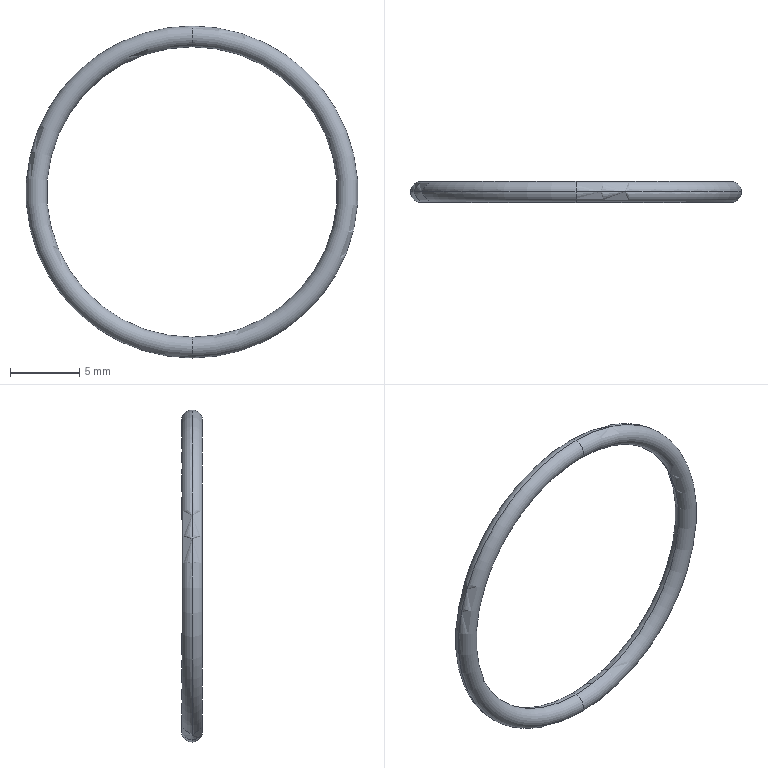Part | SolidWorks | features Revolution 1 | 1 solid | 4 faces | box 24 x 1.5 x 24 mm | volume 124.912 mm3 | torus 4
STEP:
#1=CARTESIAN_POINT('',(0.,0.,12.));
#2=VERTEX_POINT('',#1);
#3=CARTESIAN_POINT('',(0.,0.,10.5));
#4=VERTEX_POINT('',#3);
#5=CARTESIAN_POINT('',(0.,0.,11.25));
#6=DIRECTION('',(1.,0.,0.));
#7=DIRECTION('',(0.,0.,-1.));
#8=AXIS2_PLACEMENT_3D('',#5,#6,#7);
#9=CIRCLE('',#8,0.75);
#10=EDGE_CURVE('',#2,#4,#9,.T.);
#11=ORIENTED_EDGE('',*,*,#10,.F.);
#12=CARTESIAN_POINT('',(0.,0.,-12.));
#13=VERTEX_POINT('',#12);
#14=CARTESIAN_POINT('',(0.,0.,0.));
#15=DIRECTION('',(0.,-1.,0.));
#16=DIRECTION('',(0.,0.,-1.));
#17=AXIS2_PLACEMENT_3D('',#14,#15,#16);
#18=CIRCLE('',#17,12.);
#19=EDGE_CURVE('',#2,#13,#18,.T.);
#20=ORIENTED_EDGE('',*,*,#19,.T.);
#21=CARTESIAN_POINT('',(0.,0.,-10.5));
#22=VERTEX_POINT('',#21);
#23=CARTESIAN_POINT('',(0.,0.,-11.25));
#24=DIRECTION('',(-1.,0.,0.));
#25=DIRECTION('',(0.,0.,1.));
#26=AXIS2_PLACEMENT_3D('',#23,#24,#25);
#27=CIRCLE('',#26,0.75);
#28=EDGE_CURVE('',#13,#22,#27,.T.);
#29=ORIENTED_EDGE('',*,*,#28,.T.);
#30=CARTESIAN_POINT('',(0.,0.,0.));
#31=DIRECTION('',(0.,-1.,0.));
#32=DIRECTION('',(0.,0.,-1.));
#33=AXIS2_PLACEMENT_3D('',#30,#31,#32);
#34=CIRCLE('',#33,10.5);
#35=EDGE_CURVE('',#4,#22,#34,.T.);
#36=ORIENTED_EDGE('',*,*,#35,.F.);
#37=EDGE_LOOP('',(#11,#20,#29,#36));
#38=FACE_OUTER_BOUND('',#37,.T.);
#39=CARTESIAN_POINT('',(0.,0.,0.));
#40=DIRECTION('',(0.,-1.,0.));
#41=DIRECTION('',(0.,0.,-1.));
#42=AXIS2_PLACEMENT_3D('',#39,#40,#41);
#43=TOROIDAL_SURFACE('',#42,11.25,0.75);
#44=ADVANCED_FACE('',(#38),#43,.T.);
#45=ORIENTED_EDGE('',*,*,#28,.F.);
#46=CARTESIAN_POINT('',(0.,0.,0.));
#47=DIRECTION('',(0.,-1.,0.));
#48=DIRECTION('',(0.,0.,-1.));
#49=AXIS2_PLACEMENT_3D('',#46,#47,#48);
#50=CIRCLE('',#49,12.);
#51=EDGE_CURVE('',#13,#2,#50,.T.);
#52=ORIENTED_EDGE('',*,*,#51,.T.);
#53=ORIENTED_EDGE('',*,*,#10,.T.);
#54=CARTESIAN_POINT('',(0.,0.,0.));
#55=DIRECTION('',(0.,-1.,0.));
#56=DIRECTION('',(0.,0.,-1.));
#57=AXIS2_PLACEMENT_3D('',#54,#55,#56);
#58=CIRCLE('',#57,10.5);
#59=EDGE_CURVE('',#22,#4,#58,.T.);
#60=ORIENTED_EDGE('',*,*,#59,.F.);
#61=EDGE_LOOP('',(#45,#52,#53,#60));
#62=FACE_OUTER_BOUND('',#61,.T.);
#63=CARTESIAN_POINT('',(0.,0.,0.));
#64=DIRECTION('',(0.,-1.,0.));
#65=DIRECTION('',(0.,0.,-1.));
#66=AXIS2_PLACEMENT_3D('',#63,#64,#65);
#67=TOROIDAL_SURFACE('',#66,11.25,0.75);
#68=ADVANCED_FACE('',(#62),#67,.T.);
#69=ORIENTED_EDGE('',*,*,#51,.F.);
#70=CARTESIAN_POINT('',(0.,0.,-11.25));
#71=DIRECTION('',(-1.,0.,0.));
#72=DIRECTION('',(0.,0.,1.));
#73=AXIS2_PLACEMENT_3D('',#70,#71,#72);
#74=CIRCLE('',#73,0.75);
#75=EDGE_CURVE('',#22,#13,#74,.T.);
#76=ORIENTED_EDGE('',*,*,#75,.F.);
#77=ORIENTED_EDGE('',*,*,#59,.T.);
#78=CARTESIAN_POINT('',(0.,0.,11.25));
#79=DIRECTION('',(1.,0.,0.));
#80=DIRECTION('',(0.,0.,-1.));
#81=AXIS2_PLACEMENT_3D('',#78,#79,#80);
#82=CIRCLE('',#81,0.75);
#83=EDGE_CURVE('',#4,#2,#82,.T.);
#84=ORIENTED_EDGE('',*,*,#83,.T.);
#85=EDGE_LOOP('',(#69,#76,#77,#84));
#86=FACE_OUTER_BOUND('',#85,.T.);
#87=CARTESIAN_POINT('',(0.,0.,0.));
#88=DIRECTION('',(0.,-1.,0.));
#89=DIRECTION('',(0.,0.,-1.));
#90=AXIS2_PLACEMENT_3D('',#87,#88,#89);
#91=TOROIDAL_SURFACE('',#90,11.25,0.75);
#92=ADVANCED_FACE('',(#86),#91,.T.);
#93=ORIENTED_EDGE('',*,*,#19,.F.);
#94=ORIENTED_EDGE('',*,*,#83,.F.);
#95=ORIENTED_EDGE('',*,*,#35,.T.);
#96=ORIENTED_EDGE('',*,*,#75,.T.);
#97=EDGE_LOOP('',(#93,#94,#95,#96));
#98=FACE_OUTER_BOUND('',#97,.T.);
#99=CARTESIAN_POINT('',(0.,0.,0.));
#100=DIRECTION('',(0.,-1.,0.));
#101=DIRECTION('',(0.,0.,-1.));
#102=AXIS2_PLACEMENT_3D('',#99,#100,#101);
#103=TOROIDAL_SURFACE('',#102,11.25,0.75);
#104=ADVANCED_FACE('',(#98),#103,.T.);
#105=CLOSED_SHELL('',(#44,#68,#92,#104));
#106=MANIFOLD_SOLID_BREP('',#105);
#107=CARTESIAN_POINT('',(0.,0.,0.));
#108=DIRECTION('',(0.,0.,1.));
#109=DIRECTION('',(1.,0.,0.));
#110=AXIS2_PLACEMENT_3D('',#107,#108,#109);
#111=(LENGTH_UNIT()NAMED_UNIT(*)SI_UNIT(.MILLI.,.METRE.));
#112=UNCERTAINTY_MEASURE_WITH_UNIT(LENGTH_MEASURE(0.00001),#111,'','');
#113=(NAMED_UNIT(*)PLANE_ANGLE_UNIT()SI_UNIT($,.RADIAN.));
#114=(NAMED_UNIT(*)SI_UNIT($,.STERADIAN.)SOLID_ANGLE_UNIT());
#115=(GEOMETRIC_REPRESENTATION_CONTEXT(3)GLOBAL_UNCERTAINTY_ASSIGNED_CONTEXT((#112))GLOBAL_UNIT_ASSIGNED_CONTEXT((#111,#113,#114))REPRESENTATION_CONTEXT('',''));
#116=ADVANCED_BREP_SHAPE_REPRESENTATION('',(#106,#110),#115);